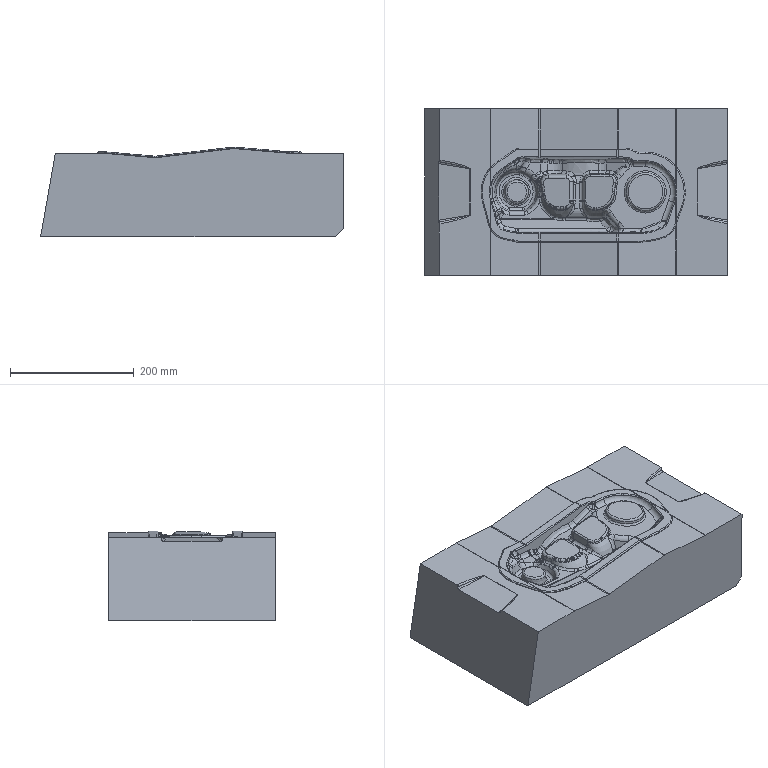NC program | NX | posted with a generic post | part box 490.523 x 270 x 145.452 mm
Lines 1 to 1174 of 9461:
N10 G17 G21 G94 G90
(ZLEVEL_PROFILE , TOOL : 25.)
N12 T00 M6
N14 G54
N16 G17 G0 G90 X-502.984 Y-55.424 S3000 M3
N18 G43 Z100. H0
N20 Z11.048
N22 G94 G1 Z9.849 F2500.
N24 X-476.828 Y0.096
N26 Y269.904
N28 X-476.917 Y269.992 Z9.35
N30 Y0.008
N32 X-477.006 Y-0.08 Z8.85
N34 Y270.08
N36 X-477.094 Y270.169 Z8.351
N38 Y-0.169
N40 X-477.182 Y-0.257 Z7.851
N42 Y270.257
N44 X-477.27 Y270.345 Z7.352
N46 Y-0.345
N48 X-477.358 Y-0.433 Z6.852
N50 Y270.433
N52 X-477.446 Y270.522 Z6.353
N54 Y-0.522
N56 X-477.534 Y-0.61 Z5.853
N58 Y270.61
N60 X-477.622 Y270.698 Z5.354
N62 Y-0.698
N64 X-477.71 Y-0.786 Z4.854
N66 Y270.786
N68 X-477.798 Y270.874 Z4.355
N70 Y-0.874
N72 X-477.886 Y-0.911 Z3.855
N74 Y270.911
N76 X-477.931 Z3.606
N78 X-477.975 Z3.356
N80 Y-0.911
N82 X-478.02 Z3.106
N84 X-478.063 Z2.856
N86 Y270.899
N88 Y270.911
N90 X-478.108 Z2.607
N92 X-478.151 Z2.357
N94 Y270.901
N96 Y-0.911
N98 X-478.196 Z2.107
N100 X-478.239 Z1.857
N102 Y270.911
N104 X-478.284 Z1.608
N106 X-478.327 Z1.358
N108 Y-0.911
N110 X-478.372 Z1.108
N112 X-478.415 Z0.858
N114 Y270.911
N116 X-478.46 Z0.609
N118 X-478.503 Z0.359
N120 Y-0.911
N122 X-478.548 Z0.109
N124 X-478.591 Z-0.141
N126 Y270.911
N128 X-478.636 Z-0.39
N130 X-478.679 Z-0.64
N132 Y-0.911
N134 X-478.724 Z-0.89
N136 X-478.767 Z-1.139
N138 Y270.911
N140 X-478.812 Z-1.389
N142 X-478.855 Z-1.639
N144 Y270.909
N146 Y-0.909
N148 Y-0.911
N150 X-478.9 Z-1.889
N152 X-478.943 Z-2.138
N154 Y270.911
N156 X-478.988 Z-2.388
N158 X-479.031 Z-2.638
N160 Y-0.911
N162 X-479.076 Z-2.888
N164 X-479.119 Z-3.137
N166 Y270.911
N168 X-479.164 Z-3.387
N170 X-479.208 Z-3.637
N172 Y-0.911
N174 X-479.253 Z-3.887
N176 X-479.296 Z-4.136
N178 Y270.911
N180 X-479.341 Z-4.386
N182 X-479.384 Z-4.636
N184 Y270.899
N186 Y-0.899
N188 Y-0.911
N190 X-479.429 Z-4.886
N192 X-479.472 Z-5.135
N194 Y270.911
N196 X-479.517 Z-5.385
N198 X-479.56 Z-5.635
N200 Y-0.911
N202 X-479.605 Z-5.885
N204 X-479.648 Z-6.134
N206 Y270.911
N208 X-479.693 Z-6.384
N210 X-479.736 Z-6.634
N212 Y-0.911
N214 X-479.781 Z-6.884
N216 X-479.824 Z-7.133
N218 Y270.911
N220 X-479.869 Z-7.383
N222 X-479.912 Z-7.633
N224 Y-0.911
N226 X-479.957 Z-7.883
N228 X-480. Z-8.132
N230 Y270.911
N232 X-480.045 Z-8.382
N234 X-480.088 Z-8.632
N236 Y270.908
N238 Y-0.908
N240 Y-0.911
N242 X-480.133 Z-8.881
N244 X-480.176 Z-9.131
N246 Y-0.909
N248 Y270.909
N250 Y270.911
N252 X-480.221 Z-9.381
N254 X-480.264 Z-9.631
N256 Y-0.911
N258 X-480.309 Z-9.88
N260 X-480.352 Z-10.13
N262 Y270.911
N264 X-480.397 Z-10.38
N266 X-480.441 Z-10.63
N268 Y-0.911
N270 X-480.486 Z-10.879
N272 X-480.529 Z-11.129
N274 Y270.911
N276 X-480.574 Z-11.379
N278 X-480.617 Z-11.629
N280 Y270.898
N282 Y-0.898
N284 Y-0.911
N286 X-480.662 Z-11.878
N288 X-480.705 Z-12.128
N290 Y270.911
N292 X-480.75 Z-12.378
N294 X-480.793 Z-12.628
N296 Y-0.911
N298 X-480.838 Z-12.877
N300 X-480.881 Z-13.127
N302 Y270.911
N304 X-480.926 Z-13.377
N306 X-480.969 Z-13.627
N308 Y-0.911
N310 X-481.014 Z-13.876
N312 X-481.057 Z-14.126
N314 Y270.911
N316 X-481.102 Z-14.376
N318 X-481.145 Z-14.626
N320 Y-0.911
N322 X-481.19 Z-14.875
N324 X-481.233 Z-15.125
N326 Y270.911
N328 X-481.278 Z-15.375
N330 X-481.321 Z-15.624
N332 Y-0.909
N334 Y-0.911
N336 X-481.366 Z-15.874
N338 X-481.409 Z-16.124
N340 Y-0.907
N342 Y270.907
N344 Y270.911
N346 X-481.454 Z-16.374
N348 X-481.497 Z-16.623
N350 Y-0.911
N352 X-481.542 Z-16.873
N354 X-481.585 Z-17.123
N356 Y270.911
N358 X-481.63 Z-17.373
N360 X-481.674 Z-17.622
N362 Y-0.911
N364 X-481.719 Z-17.872
N366 X-481.762 Z-18.122
N368 Y-0.901
N370 Y270.901
N372 Y270.911
N374 X-481.807 Z-18.372
N376 X-481.85 Z-18.621
N378 Y-0.911
N380 X-481.895 Z-18.871
N382 X-481.938 Z-19.121
N384 Y270.911
N386 X-481.983 Z-19.371
N388 X-482.026 Z-19.62
N390 Y-0.911
N392 X-482.071 Z-19.87
N394 X-482.114 Z-20.12
N396 Y270.911
N398 X-482.159 Z-20.37
N400 X-482.202 Z-20.619
N402 Y-0.911
N404 X-482.247 Z-20.869
N406 X-482.29 Z-21.119
N408 Y270.911
N410 X-482.335 Z-21.369
N412 X-482.378 Z-21.618
N414 Y-0.911
N416 X-482.423 Z-21.868
N418 X-482.466 Z-22.118
N420 Y270.911
N422 X-482.511 Z-22.367
N424 X-482.554 Z-22.617
N426 Y-0.911
N428 X-482.599 Z-22.867
N430 X-482.642 Z-23.117
N432 Y-0.905
N434 Y270.905
N436 Y270.911
N438 X-482.687 Z-23.366
N440 X-482.73 Z-23.616
N442 Y270.902
N444 Y-0.899
N446 Y-0.911
N448 X-482.775 Z-23.866
N450 X-482.818 Z-24.116
N452 Y270.911
N454 X-482.863 Z-24.365
N456 X-482.907 Z-24.615
N458 Y-0.911
N460 X-482.952 Z-24.865
N462 X-482.995 Z-25.115
N464 Y270.911
N466 X-483.04 Z-25.364
N468 X-483.083 Z-25.614
N470 Y-0.911
N472 X-483.128 Z-25.864
N474 X-483.171 Z-26.114
N476 Y270.911
N478 X-483.216 Z-26.363
N480 X-483.259 Z-26.613
N482 Y-0.911
N484 X-483.304 Z-26.863
N486 X-483.347 Z-27.113
N488 Y270.911
N490 X-483.392 Z-27.362
N492 X-483.435 Z-27.612
N494 Y-0.911
N496 X-483.48 Z-27.862
N498 X-483.523 Z-28.112
N500 Y270.911
N502 X-483.568 Z-28.361
N504 X-483.611 Z-28.611
N506 Y-0.91
N508 X-483.656 Y-0.911 Z-28.861
N510 X-483.699 Z-29.11
N512 Y270.911
N514 X-483.744 Z-29.36
N516 X-483.787 Z-29.61
N518 Y270.902
N520 Y-0.902
N522 Y-0.911
N524 X-483.832 Z-29.86
N526 X-483.875 Z-30.109
N528 Y-0.904
N530 Y270.904
N532 Y270.911
N534 X-483.92 Z-30.359
N536 X-483.963 Z-30.609
N538 Y270.901
N540 Y-0.9
N542 Y-0.911
N544 X-484.008 Z-30.859
N546 X-484.051 Z-31.108
N548 Y270.911
N550 X-484.096 Z-31.358
N552 X-484.14 Z-31.608
N554 Y-0.911
N556 X-484.185 Z-31.858
N558 X-484.228 Z-32.107
N560 Y270.911
N562 X-484.273 Z-32.357
N564 X-484.316 Z-32.607
N566 Y-0.911
N568 X-484.361 Z-32.857
N570 X-484.404 Z-33.106
N572 Y270.911
N574 X-484.449 Z-33.356
N576 X-484.492 Z-33.606
N578 Y-0.911
N580 X-484.537 Z-33.856
N582 X-484.58 Z-34.105
N584 Y270.911
N586 X-484.625 Z-34.355
N588 X-484.668 Z-34.605
N590 Y-0.911
N592 X-484.713 Z-34.855
N594 X-484.756 Z-35.104
N596 Y-0.91
N598 Y270.91
N600 Y270.911
N602 X-484.801 Z-35.354
N604 X-484.844 Z-35.604
N606 Y-0.91
N608 X-484.889 Y-0.911 Z-35.854
N610 X-484.932 Z-36.103
N612 Y270.911
N614 X-484.977 Z-36.353
N616 X-485.02 Z-36.603
N618 Y-0.911
N620 X-485.065 Z-36.852
N622 X-485.108 Z-37.102
N624 Y-0.902
N626 Y270.902
N628 Y270.911
N630 X-485.153 Z-37.352
N632 X-485.196 Z-37.602
N634 Y270.9
N636 Y-0.901
N638 Y-0.911
N640 X-485.241 Z-37.851
N642 X-485.284 Z-38.101
N644 Y270.911
N646 X-485.329 Z-38.351
N648 X-485.373 Z-38.601
N650 Y-0.911
N652 X-485.418 Z-38.85
N654 X-485.461 Z-39.1
N656 Y270.911
N658 X-485.506 Z-39.35
N660 X-485.549 Z-39.6
N662 Y-0.911
N664 X-485.594 Z-39.849
N666 X-485.637 Z-40.099
N668 Y270.911
N670 X-485.682 Z-40.349
N672 X-485.725 Z-40.599
N674 Y-0.911
N676 X-485.77 Z-40.848
N678 X-485.813 Z-41.098
N680 Y270.911
N682 X-485.858 Z-41.348
N684 X-485.901 Z-41.598
N686 Y-0.911
N688 X-485.946 Z-41.847
N690 X-485.989 Z-42.097
N692 Y-0.91
N694 Y270.91
N696 Y270.911
N698 X-486.034 Z-42.347
N700 X-486.077 Z-42.597
N702 Y-0.911
N704 X-486.122 Z-42.846
N706 X-486.165 Z-43.096
N708 Y270.911
N710 X-486.21 Z-43.346
N712 X-486.253 Z-43.595
N714 Y270.91
N716 Y-0.91
N718 Y-0.911
N720 X-486.298 Z-43.845
N722 X-486.341 Z-44.095
N724 Y-0.901
N726 Y270.901
N728 Y270.911
N730 X-486.386 Z-44.345
N732 X-486.429 Z-44.594
N734 Y270.901
N736 Y-0.902
N738 Y-0.911
N740 X-486.474 Z-44.844
N742 X-486.518 Z-45.094
N744 Y270.911
N746 X-486.563 Z-45.344
N748 X-486.606 Z-45.593
N750 Y-0.911
N752 X-486.651 Z-45.843
N754 X-486.694 Z-46.093
N756 Y270.911
N758 X-486.739 Z-46.343
N760 X-486.782 Z-46.592
N762 Y-0.911
N764 X-486.827 Z-46.842
N766 X-486.87 Z-47.092
N768 Y270.911
N770 X-486.915 Z-47.342
N772 X-486.958 Z-47.591
N774 Y-0.911
N776 X-487.003 Z-47.841
N778 X-487.046 Z-48.091
N780 Y-0.895
N782 Y270.895
N784 Y270.911
N786 X-487.091 Z-48.341
N788 X-487.134 Z-48.59
N790 Y-0.911
N792 X-487.179 Z-48.84
N794 X-487.222 Z-49.09
N796 Y-0.91
N798 Y270.91
N800 Y270.911
N802 X-487.267 Z-49.34
N804 X-487.31 Z-49.589
N806 Y-0.911
N808 X-487.355 Z-49.839
N810 X-487.398 Z-50.089
N812 Y270.911
N814 X-487.443 Z-50.338
N816 X-487.486 Z-50.588
N818 Y270.908
N820 Y-0.908
N822 Y-0.911
N824 X-487.531 Z-50.838
N826 X-487.574 Z-51.088
N828 Y-0.9
N830 Y270.9
N832 Y270.911
N834 X-487.619 Z-51.337
N836 X-487.662 Z-51.587
N838 Y-0.911
N840 X-487.707 Z-51.837
N842 X-487.751 Z-52.087
N844 Y270.911
N846 X-487.796 Z-52.336
N848 X-487.839 Z-52.586
N850 Y-0.911
N852 X-487.884 Z-52.836
N854 X-487.927 Z-53.086
N856 Y270.911
N858 X-487.972 Z-53.335
N860 X-488.015 Z-53.585
N862 Y-0.911
N864 X-488.06 Z-53.835
N866 X-488.103 Z-54.085
N868 Y270.911
N870 X-488.148 Z-54.334
N872 X-488.191 Z-54.584
N874 Y270.905
N876 Y-0.905
N878 Y-0.911
N880 X-488.236 Z-54.834
N882 X-488.279 Z-55.084
N884 Y-0.895
N886 Y270.895
N888 Y270.911
N890 X-488.324 Z-55.333
N892 X-488.367 Z-55.583
N894 Y-0.911
N896 X-488.412 Z-55.833
N898 X-488.455 Z-56.083
N900 Y-0.91
N902 Y270.91
N904 Y270.911
N906 X-488.5 Z-56.332
N908 X-488.543 Z-56.582
N910 Y-0.911
N912 X-488.588 Z-56.832
N914 X-488.631 Z-57.081
N916 Y-0.902
N918 Y270.902
N920 Y270.911
N922 X-488.676 Z-57.331
N924 X-488.719 Z-57.581
N926 Y270.906
N928 Y-0.906
N930 Y-0.911
N932 X-488.764 Z-57.831
N934 X-488.807 Z-58.08
N936 Y-0.898
N938 Y270.901
N940 Y270.911
N942 X-488.852 Z-58.33
N944 X-488.895 Z-58.58
N946 Y-0.911
N948 X-488.94 Z-58.83
N950 X-488.984 Z-59.079
N952 Y270.911
N954 X-489.029 Z-59.329
N956 X-489.072 Z-59.579
N958 Y-0.911
N960 X-489.117 Z-59.829
N962 X-489.16 Z-60.078
N964 Y270.911
N966 X-489.205 Z-60.328
N968 X-489.248 Z-60.578
N970 Y-0.911
N972 X-489.293 Z-60.828
N974 X-489.336 Z-61.077
N976 Y270.911
N978 X-489.381 Z-61.327
N980 X-489.424 Z-61.577
N982 Y270.905
N984 Y-0.905
N986 Y-0.911
N988 X-489.469 Z-61.827
N990 X-489.512 Z-62.076
N992 Y-0.894
N994 Y270.894
N996 Y270.911
N998 X-489.557 Z-62.326
N1000 X-489.6 Z-62.576
N1002 Y270.895
N1004 Y-0.895
N1006 Y-0.911
N1008 X-489.645 Z-62.826
N1010 X-489.688 Z-63.075
N1012 Y270.91
N1014 X-489.733 Y270.911 Z-63.325
N1016 X-489.776 Z-63.575
N1018 Y-0.911
N1020 X-489.821 Z-63.824
N1022 X-489.864 Z-64.074
N1024 Y-0.901
N1026 Y270.901
N1028 Y270.911
N1030 X-489.909 Z-64.324
N1032 X-489.952 Z-64.574
N1034 Y270.903
N1036 Y-0.903
N1038 Y-0.911
N1040 X-489.997 Z-64.823
N1042 X-490.04 Z-65.073
N1044 Y-0.9
N1046 Y270.9
N1048 Y270.911
N1050 X-490.085 Z-65.323
N1052 X-490.128 Z-65.573
N1054 Y-0.911
N1056 X-490.173 Z-65.822
N1058 X-490.217 Z-66.072
N1060 Y270.911
N1062 X-490.262 Z-66.322
N1064 X-490.305 Z-66.572
N1066 Y-0.911
N1068 X-490.35 Z-66.821
N1070 X-490.393 Z-67.071
N1072 Y270.911
N1074 X-490.438 Z-67.321
N1076 X-490.481 Z-67.571
N1078 Y-0.911
N1080 X-490.526 Z-67.82
N1082 X-490.569 Z-68.07
N1084 Y270.911
N1086 X-490.614 Z-68.32
N1088 X-490.657 Z-68.57
N1090 Y270.895
N1092 Y-0.895
N1094 Y-0.911
N1096 X-490.702 Z-68.819
N1098 X-490.745 Z-69.069
N1100 Y-0.893
N1102 Y270.893
N1104 Y270.911
N1106 X-490.79 Z-69.319
N1108 X-490.833 Z-69.569
N1110 Y-0.911
N1112 X-490.878 Z-69.818
N1114 X-490.921 Z-70.068
N1116 Y270.911
N1118 X-490.966 Z-70.318
N1120 X-491.009 Z-70.568
N1122 Y-0.911
N1124 X-491.054 Z-70.817
N1126 X-491.097 Z-71.067
N1128 Y270.91
N1130 Y270.911
N1132 X-491.142 Z-71.317
N1134 X-491.185 Z-71.566
N1136 Y270.901
N1138 Y-0.901
N1140 Y-0.911
N1142 X-491.23 Z-71.816
N1144 X-491.273 Z-72.066
N1146 Y-0.901
N1148 Y270.9
N1150 Y270.911
N1152 X-491.318 Z-72.316
N1154 X-491.361 Z-72.565
N1156 Y-0.911
N1158 X-491.406 Z-72.815
N1160 X-491.45 Z-73.065
N1162 Y270.911
N1164 X-491.495 Z-73.315
N1166 X-491.538 Z-73.564
N1168 Y-0.911
N1170 X-491.583 Z-73.814
N1172 X-491.626 Z-74.064
N1174 Y270.911
N1176 X-491.671 Z-74.314
N1178 X-491.714 Z-74.563
N1180 Y-0.911
N1182 X-491.759 Z-74.813
N1184 X-491.802 Z-75.063
N1186 Y270.911
N1188 X-491.847 Z-75.313
N1190 X-491.89 Z-75.562
N1192 Y270.895
N1194 Y-0.895
N1196 Y-0.911
N1198 X-491.935 Z-75.812
N1200 X-491.978 Z-76.062
N1202 Y270.911
N1204 X-492.023 Z-76.312
N1206 X-492.066 Z-76.561
N1208 Y-0.911
N1210 X-492.111 Z-76.811
N1212 X-492.154 Z-77.061
N1214 Y270.911
N1216 X-492.199 Z-77.311
N1218 X-492.242 Z-77.56
N1220 Y-0.911
N1222 X-492.287 Z-77.81
N1224 X-492.33 Z-78.06
N1226 Y-0.909
N1228 Y270.908
N1230 Y270.911
N1232 X-492.375 Z-78.309
N1234 X-492.418 Z-78.559
N1236 Y270.9
N1238 Y-0.9
N1240 Y-0.911
N1242 X-492.463 Z-78.809
N1244 X-492.506 Z-79.059
N1246 Y270.911
N1248 X-492.551 Z-79.308
N1250 X-492.594 Z-79.558
N1252 Y-0.911
N1254 X-492.639 Z-79.808
N1256 X-492.683 Z-80.058
N1258 Y270.911
N1260 X-492.728 Z-80.307
N1262 X-492.771 Z-80.557
N1264 Y-0.911
N1266 X-492.816 Z-80.807
N1268 X-492.859 Z-81.057
N1270 Y270.911
N1272 X-492.904 Z-81.306
N1274 X-492.947 Z-81.556
N1276 Y-0.911
N1278 X-492.992 Z-81.806
N1280 X-493.035 Z-82.056
N1282 Y270.911
N1284 X-493.08 Z-82.305
N1286 X-493.123 Z-82.555
N1288 Y270.895
N1290 Y-0.895
N1292 Y-0.911
N1294 X-493.168 Z-82.805
N1296 X-493.211 Z-83.055
N1298 Y270.911
N1300 X-493.256 Z-83.304
N1302 X-493.299 Z-83.554
N1304 Y-0.911
N1306 X-493.344 Z-83.804
N1308 X-493.387 Z-84.054
N1310 Y270.911
N1312 X-493.432 Z-84.303
N1314 X-493.475 Z-84.553
N1316 Y270.902
N1318 Y-0.911
N1320 X-493.52 Z-84.803
N1322 X-493.563 Z-85.052
N1324 Y-0.907
N1326 Y270.907
N1328 Y270.911
N1330 X-493.608 Z-85.302
N1332 X-493.651 Z-85.552
N1334 Y270.899
N1336 Y-0.899
N1338 Y-0.911
N1340 X-493.696 Z-85.802
N1342 X-493.739 Z-86.051
N1344 Y270.911
N1346 X-493.784 Z-86.301
N1348 X-493.827 Z-86.551
N1350 Y-0.911
N1352 X-493.872 Z-86.801
N1354 X-493.916 Z-87.05
N1356 Y270.911
N1358 X-493.961 Z-87.3
N1360 X-494.004 Z-87.55
N1362 Y-0.911
N1364 X-494.049 Z-87.8
N1366 X-494.092 Z-88.049
N1368 Y270.911
N1370 X-494.137 Z-88.299
N1372 X-494.18 Z-88.549
N1374 Y-0.911
N1376 X-494.225 Z-88.799
N1378 X-494.268 Z-89.048
N1380 Y-0.905
N1382 Y270.905
N1384 Y270.911
N1386 X-494.313 Z-89.298
N1388 X-494.356 Z-89.548
N1390 Y270.895
N1392 Y-0.895
N1394 Y-0.911
N1396 X-494.401 Z-89.798
N1398 X-494.444 Z-90.047
N1400 Y270.911
N1402 X-494.489 Z-90.297
N1404 X-494.532 Z-90.547
N1406 Y-0.911
N1408 X-494.577 Z-90.797
N1410 X-494.62 Y-0.912 Z-91.046
N1412 Y270.912
N1414 X-494.665 Y270.911 Z-91.296
N1416 X-494.708 Z-91.546
N1418 Y270.902
N1420 Y-0.901
N1422 Y-0.911
N1424 X-494.753 Z-91.795
N1426 X-494.796 Z-92.045
N1428 Y-0.903
N1430 Y270.903
N1432 Y270.911
N1434 X-494.841 Z-92.295
N1436 X-494.884 Z-92.545
N1438 Y270.901
N1440 Y-0.9
N1442 Y-0.911
N1444 X-494.929 Z-92.794
N1446 X-494.972 Z-93.044
N1448 Y270.911
N1450 X-495.017 Z-93.294
N1452 X-495.061 Z-93.544
N1454 Y-0.911
N1456 X-495.106 Z-93.793
N1458 X-495.149 Z-94.043
N1460 Y270.911
N1462 X-495.194 Z-94.293
N1464 X-495.237 Z-94.543
N1466 Y-0.911
N1468 X-495.282 Z-94.792
N1470 X-495.325 Z-95.042
N1472 Y270.911
N1474 X-495.37 Z-95.292
N1476 X-495.413 Z-95.542
N1478 Y-0.911
N1480 X-495.458 Z-95.791
N1482 X-495.501 Z-96.041
N1484 Y-0.896
N1486 Y270.896
N1488 Y270.911
N1490 X-495.546 Z-96.291
N1492 X-495.589 Z-96.541
N1494 Y270.893
N1496 Y-0.893
N1498 Y-0.911
N1500 X-495.634 Z-96.79
N1502 X-495.677 Z-97.04
N1504 Y270.911
N1506 X-495.722 Z-97.29
N1508 X-495.765 Z-97.54
N1510 Y270.91
N1512 Y-0.91
N1514 Y-0.911
N1516 X-495.81 Z-97.789
N1518 X-495.853 Z-98.039
N1520 Y270.911
N1522 X-495.898 Z-98.289
N1524 X-495.941 Z-98.539
N1526 Y-0.911
N1528 X-495.986 Z-98.788
N1530 X-496.029 Z-99.038
N1532 Y-0.902
N1534 Y270.902
N1536 Y270.911
N1538 X-496.074 Z-99.288
N1540 X-496.117 Z-99.537
N1542 Y270.9
N1544 Y-0.901
N1546 Y-0.911
N1548 X-496.162 Z-99.787
N1550 X-496.205 Z-100.037
N1552 Y270.911
N1554 X-496.25 Z-100.287
N1556 X-496.294 Z-100.536
N1558 Y-0.911
N1560 X-496.339 Z-100.786
N1562 X-496.382 Z-101.036
N1564 Y270.911
N1566 X-496.427 Z-101.286
N1568 X-496.47 Z-101.535
N1570 Y-0.911
N1572 X-496.515 Z-101.785
N1574 X-496.558 Z-102.035
N1576 Y270.911
N1578 X-496.603 Z-102.285
N1580 X-496.646 Z-102.534
N1582 Y-0.911
N1584 X-496.691 Z-102.784
N1586 X-496.734 Z-103.034
N1588 Y-0.895
N1590 Y270.895
N1592 Y270.911
N1594 X-496.779 Z-103.284
N1596 X-496.822 Z-103.533
N1598 Y-0.911
N1600 X-496.867 Z-103.783
N1602 X-496.91 Z-104.033
N1604 Y270.911
N1606 X-496.955 Z-104.283
N1608 X-496.998 Z-104.532
N1610 Y-0.911
N1612 X-497.043 Z-104.782
N1614 X-497.086 Z-105.032
N1616 Y270.911
N1618 X-497.131 Z-105.282
N1620 X-497.174 Z-105.531
N1622 Y270.909
N1624 Y-0.909
N1626 Y-0.911
N1628 X-497.219 Z-105.781
N1630 X-497.262 Z-106.031
N1632 Y-0.901
N1634 Y270.901
N1636 Y270.911
N1638 X-497.307 Z-106.28
N1640 X-497.35 Z-106.53
N1642 Y270.901
N1644 Y-0.911
N1646 X-497.395 Z-106.78
N1648 X-497.438 Z-107.03
N1650 Y270.911
N1652 X-497.483 Z-107.279
N1654 X-497.527 Z-107.529
N1656 Y-0.911
N1658 X-497.572 Z-107.779
N1660 X-497.615 Z-108.029
N1662 Y270.911
N1664 X-497.66 Z-108.278
N1666 X-497.703 Z-108.528
N1668 Y-0.911
N1670 X-497.748 Z-108.778
N1672 X-497.791 Z-109.028
N1674 Y270.911
N1676 X-497.836 Z-109.277
N1678 X-497.879 Z-109.527
N1680 Y-0.911
N1682 X-497.924 Z-109.777
N1684 X-497.967 Z-110.027
N1686 Y-0.895
N1688 Y270.895
N1690 Y270.911
N1692 X-498.012 Z-110.276
N1694 X-498.055 Z-110.526
N1696 Y-0.911
N1698 X-498.1 Z-110.776
N1700 X-498.143 Z-111.026
N1702 Y270.911
N1704 X-498.188 Z-111.275
N1706 X-498.231 Z-111.525
N1708 Y-0.911
N1710 X-498.276 Z-111.775
N1712 X-498.319 Z-112.025
N1714 Y270.911
N1716 X-498.364 Z-112.274
N1718 X-498.407 Z-112.524
N1720 Y270.908
N1722 Y-0.908
N1724 Y-0.911
N1726 X-498.452 Z-112.774
N1728 X-498.495 Z-113.023
N1730 Y-0.899
N1732 Y270.902
N1734 Y270.911
N1736 X-498.54 Z-113.273
N1738 X-498.583 Z-113.523
N1740 Y-0.911
N1742 X-498.628 Z-113.773
N1744 X-498.671 Z-114.022
N1746 Y270.911
N1748 X-498.716 Z-114.272
N1750 X-498.76 Z-114.522
N1752 Y-0.911
N1754 X-498.805 Z-114.772
N1756 X-498.848 Z-115.021
N1758 Y270.911
N1760 X-498.893 Z-115.271
N1762 X-498.936 Z-115.521
N1764 Y-0.911
N1766 X-498.981 Z-115.771
N1768 X-499.024 Z-116.02
N1770 Y270.911
N1772 X-499.069 Z-116.27
N1774 X-499.112 Z-116.52
N1776 Y270.905
N1778 Y-0.905
N1780 Y-0.911
N1782 X-499.157 Z-116.77
N1784 X-499.2 Z-117.019
N1786 Y-0.895
N1788 Y270.895
N1790 Y270.911
N1792 X-499.245 Z-117.269
N1794 X-499.288 Z-117.519
N1796 Y-0.911
N1798 X-499.333 Z-117.769
N1800 X-499.376 Z-118.018
N1802 Y270.911
N1804 X-499.421 Z-118.268
N1806 X-499.464 Z-118.518
N1808 Y-0.911
N1810 X-499.509 Z-118.768
N1812 X-499.552 Z-119.017
N1814 Y-0.902
N1816 Y270.902
N1818 Y270.911
N1820 X-499.597 Z-119.267
N1822 X-499.64 Z-119.517
N1824 Y270.904
N1826 Y-0.906
N1828 Y-0.911
N1830 X-499.685 Z-119.766
N1832 X-499.728 Z-120.016
N1834 Y-0.9
N1836 Y270.901
N1838 Y270.911
N1840 X-499.773 Z-120.266
N1842 X-499.816 Z-120.516
N1844 Y-0.911
N1846 X-499.861 Z-120.765
N1848 X-499.904 Z-121.015
N1850 Y270.911
N1852 X-499.949 Z-121.265
N1854 X-499.993 Z-121.515
N1856 Y-0.911
N1858 X-500.038 Z-121.764
N1860 X-500.081 Z-122.014
N1862 Y270.911
N1864 X-500.126 Z-122.264
N1866 X-500.169 Z-122.514
N1868 Y-0.911
N1870 X-500.214 Z-122.763
N1872 X-500.257 Z-123.013
N1874 Y270.911
N1876 X-500.302 Z-123.263
N1878 X-500.345 Z-123.513
N1880 Y270.905
N1882 Y-0.905
N1884 Y-0.911
N1886 X-500.39 Z-123.762
N1888 X-500.433 Z-124.012
N1890 Y-0.894
N1892 Y270.894
N1894 Y270.911
N1896 X-500.478 Z-124.262
N1898 X-500.521 Z-124.512
N1900 Y270.894
N1902 Y-0.911
N1904 X-500.566 Z-124.761
N1906 X-500.609 Z-125.011
N1908 Y-0.91
N1910 Y270.91
N1912 X-500.654 Y270.911 Z-125.261
N1914 X-500.697 Z-125.511
N1916 Y-0.911
N1918 X-500.742 Z-125.76
N1920 X-500.785 Z-126.01
N1922 Y-0.901
N1924 Y270.901
N1926 Y270.911
N1928 X-500.83 Z-126.26
N1930 X-500.873 Z-126.51
N1932 Y270.902
N1934 Y-0.902
N1936 Y-0.911
N1938 X-500.918 Z-126.759
N1940 X-500.961 Z-127.009
N1942 Y-0.897
N1944 Y270.9
N1946 Y270.911
N1948 X-501.006 Z-127.259
N1950 X-501.049 Z-127.508
N1952 Y-0.911
N1954 X-501.094 Z-127.758
N1956 X-501.137 Z-128.008
N1958 Y270.911
N1960 X-501.182 Z-128.258
N1962 X-501.226 Z-128.507
N1964 Y-0.911
N1966 X-501.271 Z-128.757
N1968 X-501.314 Z-129.007
N1970 Y270.911
N1972 X-501.359 Z-129.257
N1974 X-501.402 Z-129.506
N1976 Y-0.911
N1978 X-501.447 Z-129.756
N1980 X-501.49 Z-130.006
N1982 Y270.911
N1984 X-501.535 Z-130.256
N1986 X-501.578 Z-130.505
N1988 Y270.899
N1990 Y-0.898
N1992 Y-0.911
N1994 X-501.623 Z-130.755
N1996 X-501.666 Z-131.005
N1998 Y-0.895
N2000 Y270.911
N2002 X-501.711 Z-131.255
N2004 X-501.754 Z-131.504
N2006 Y-0.911
N2008 X-501.799 Z-131.754
N2010 X-501.842 Z-132.004
N2012 Y-0.906
N2014 Y270.908
N2016 Y270.911
N2018 X-501.887 Z-132.254
N2020 X-501.93 Z-132.503
N2022 Y270.901
N2024 Y-0.901
N2026 Y-0.911
N2028 X-501.975 Z-132.753
N2030 X-502.018 Z-133.003
N2032 Y-0.9
N2034 Y270.898
N2036 Y270.911
N2038 X-502.063 Y270.901 Z-133.253
N2040 X-502.106 Y270.892 Z-133.502
N2042 Y-0.892
N2044 X-502.194 Y-0.723 Z-134.002
N2046 Y270.723
N2048 X-502.282 Y270.555 Z-134.501
N2050 Y-0.555
N2052 X-502.371 Y-0.387 Z-135.001
N2054 Y270.387
N2056 X-502.457 Y270.219 Z-135.5
N2058 Y-0.219
N2060 X-502.545 Y-0.05 Z-136.
N2062 Y270.05
N2064 Z-129.75
N2066 G0 Z100.
(CAVITY_MILL , TOOL : 25.)
N2068 X-294.175 Y282.5
N2070 Z10.155
N2072 G1 Z9.955
N2074 Y270.
N2076 X0.
N2078 Y0.
N2080 X-464.459
N2082 Y270.
N2084 X-294.175
N2086 Y254.79
N2088 X-15.21
N2090 Y15.21
N2092 X-449.249
N2094 Y254.79
N2096 X-294.175
N2098 Y239.58
N2100 X-30.42
N2102 Y30.42
N2104 X-434.039
N2106 Y239.58
N2108 X-294.175
N2110 Y224.37
N2112 X-45.63
N2114 Y45.63
N2116 X-160.036
N2118 G3 X-156.426 Y55.337 R15.598
N2120 G1 Y67.153
N2122 G3 X-159.994 Y76.869 R15.014
N2124 X-160.427 Y77.287 R3.042
N2126 G1 X-164.054 Y80.153
N2128 G3 X-164.568 Y80.482 R3.042
N2130 X-172.855 Y82.953 R24.399
N2132 X-187.978 Y81.082 R26.298
N2134 X-197.125 Y67.144 R15.384
N2136 G1 Y55.302
N2138 G3 X-193.609 Y45.63 R15.061
N2140 G1 X-191.277 Y47.584
N2142 G2 X-194.083 Y55.302 R12.019
N2144 G1 Y67.144
N2146 G2 X-186.746 Y78.301 R12.342
N2148 X-173.283 Y79.94 R23.256
N2150 X-165.94 Y77.767 R21.357
N2152 G1 X-162.313 Y74.9
N2154 G2 X-159.468 Y67.153 R11.972
N2156 G1 Y55.337
N2158 G2 X-168.807 Y43.474 R12.556
N2160 X-175.519 Y42.282 R41.004
N2162 X-187.56 Y44.614 R21.91
N2164 X-191.277 Y47.584 R12.019
N2166 G1 X-193.609 Y45.63
N2168 X-418.829
N2170 Y224.37
N2172 X-294.175
N2174 Y209.16
N2176 X-195.983
N2178 G3 X-197.122 Y203.867 R16.068
N2180 G1 X-197.125 Y203.737
N2182 Y191.784
N2184 G3 X-188.331 Y178.008 R15.188
N2186 X-172.844 Y175.79 R27.149
N2188 G1 X-171.636 Y175.96
N2190 X-171.56 Y175.972
N2192 X-170.336 Y176.175
N2194 G3 X-170.123 Y176.219 R3.042
N2196 G1 X-168.899 Y176.514
N2198 X-168.871 Y176.521
N2200 X-168.044 Y176.728
N2202 G3 X-156.426 Y191.481 R15.495
N2204 G1 Y203.737
N2206 G3 X-157.509 Y209.16 R15.666
N2208 G1 X-160.339 Y208.048
N2210 G2 X-159.468 Y203.737 R12.624
N2212 G1 Y191.481
N2214 G2 X-168.785 Y179.679 R12.453
N2216 G1 X-169.612 Y179.471
N2218 X-170.836 Y179.176
N2220 X-172.06 Y178.972
N2222 X-173.283 Y178.8
N2224 G2 X-187.051 Y180.767 R24.107
N2226 X-194.083 Y191.784 R12.146
N2228 G1 Y203.737
N2230 G2 X-186.144 Y215.177 R13.026
N2232 G1 X-185.522 Y215.404
N2234 G2 X-170.836 Y216.061 R24.528
N2236 G1 X-169.612 Y215.809
N2238 G2 X-160.339 Y208.048 R12.624
N2240 G1 X-157.509 Y209.16
N2242 X-60.84
N2244 Y60.84
N2246 X-141.216
N2248 Y67.153
N2250 G3 X-148.399 Y86.712 R30.224
N2252 X-150.995 Y89.219 R18.252
N2254 G1 X-154.622 Y92.086
N2256 G3 X-157.706 Y94.056 R18.252
N2258 X-170.71 Y98.015 R39.609
N2260 X-194.139 Y94.989 R41.508
N2262 X-212.335 Y67.205 R30.594
N2264 G1 Y60.84
N2266 X-403.619
N2268 Y209.16
N2270 X-294.175
N2272 Y193.95
N2274 X-212.335
N2276 Y191.784
N2278 G3 X-194.735 Y164.211 R30.398
N2280 X-170.655 Y160.738 R42.359
N2282 G1 X-169.421 Y160.912
N2284 X-169.156 Y160.952
N2286 X-167.838 Y161.172
N2288 G3 X-166.56 Y161.432 R18.252
N2290 G1 X-164.24 Y162.002
N2292 G3 X-141.216 Y191.358 R30.705
N2294 G1 Y193.95
N2296 X-76.05
N2298 Y76.05
N2300 X-126.886
N2302 G3 X-136.803 Y96.555 R45.434
N2304 X-141.564 Y101.152 R33.462
N2306 G1 X-145.191 Y104.019
N2308 G3 X-150.845 Y107.63 R33.462
N2310 X-168.562 Y113.075 R54.819
N2312 X-200.3 Y108.895 R56.718
N2314 X-226.647 Y76.05 R45.804
N2316 G1 X-388.409
N2318 Y193.95
N2320 X-294.175
N2322 Y178.74
N2324 X-225.64
N2326 G3 X-201.138 Y150.415 R45.608
N2328 X-168.479 Y145.684 R57.569
N2330 G1 X-167.206 Y145.864
N2332 X-166.752 Y145.933
N2334 X-165.339 Y146.169
N2336 G3 X-162.965 Y146.653 R33.462
N2338 G1 X-160.524 Y147.252
N2340 G3 X-127.88 Y178.74 R45.915